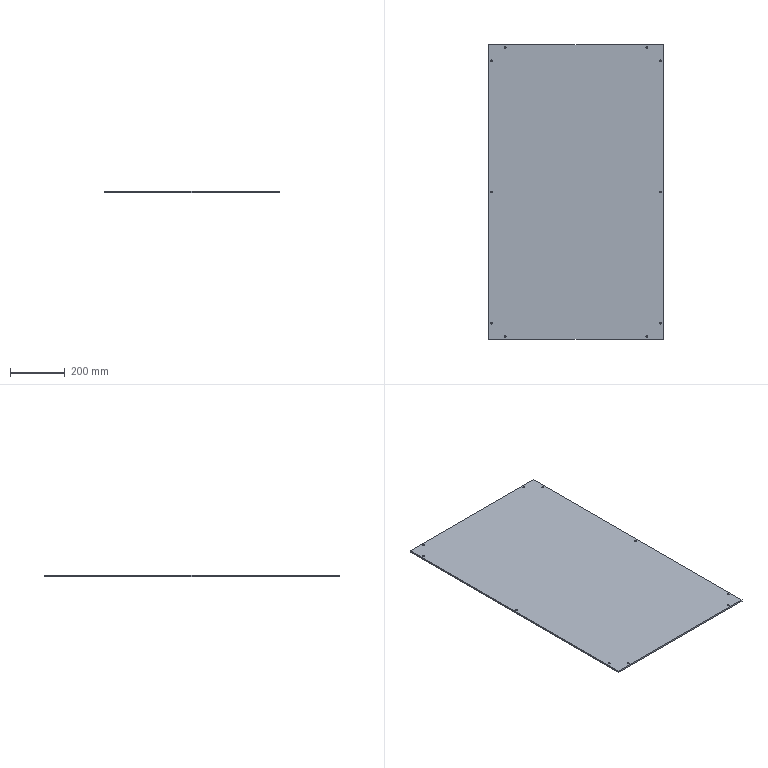Part | SolidWorks | features BaseBody 1 | 1 solid | 26 faces | box 638 x 1078 x 6 mm | volume 4124275 mm3 | cylinder 20 | plane 6 | commonest cylinder face diameters 7 x20
STEP:
#1=CARTESIAN_POINT('',(304.5,-479.,0.));
#2=VERTEX_POINT('',#1);
#3=CARTESIAN_POINT('',(311.5,-479.,0.));
#4=VERTEX_POINT('',#3);
#5=CARTESIAN_POINT('',(308.,-479.,0.));
#6=DIRECTION('',(0.,0.,1.));
#7=DIRECTION('',(1.,0.,0.));
#8=AXIS2_PLACEMENT_3D('',#5,#6,#7);
#9=CIRCLE('',#8,3.5);
#10=EDGE_CURVE('',#2,#4,#9,.T.);
#11=ORIENTED_EDGE('',*,*,#10,.F.);
#12=CARTESIAN_POINT('',(304.5,-479.,6.));
#13=VERTEX_POINT('',#12);
#14=CARTESIAN_POINT('',(304.5,-479.,6.));
#15=DIRECTION('',(0.,0.,1.));
#16=VECTOR('',#15,1000.);
#17=LINE('',#14,#16);
#18=EDGE_CURVE('',#2,#13,#17,.T.);
#19=ORIENTED_EDGE('',*,*,#18,.T.);
#20=CARTESIAN_POINT('',(311.5,-479.,6.));
#21=VERTEX_POINT('',#20);
#22=CARTESIAN_POINT('',(308.,-479.,6.));
#23=DIRECTION('',(0.,0.,1.));
#24=DIRECTION('',(1.,0.,0.));
#25=AXIS2_PLACEMENT_3D('',#22,#23,#24);
#26=CIRCLE('',#25,3.5);
#27=EDGE_CURVE('',#13,#21,#26,.T.);
#28=ORIENTED_EDGE('',*,*,#27,.T.);
#29=CARTESIAN_POINT('',(311.5,-479.,6.));
#30=DIRECTION('',(0.,0.,1.));
#31=VECTOR('',#30,1000.);
#32=LINE('',#29,#31);
#33=EDGE_CURVE('',#4,#21,#32,.T.);
#34=ORIENTED_EDGE('',*,*,#33,.F.);
#35=EDGE_LOOP('',(#11,#19,#28,#34));
#36=FACE_OUTER_BOUND('',#35,.T.);
#37=CARTESIAN_POINT('',(308.,-479.,6.));
#38=DIRECTION('',(0.,0.,1.));
#39=DIRECTION('',(1.,0.,0.));
#40=AXIS2_PLACEMENT_3D('',#37,#38,#39);
#41=CYLINDRICAL_SURFACE('',#40,3.5);
#42=ADVANCED_FACE('',(#36),#41,.F.);
#43=CARTESIAN_POINT('',(304.5,0.,0.));
#44=VERTEX_POINT('',#43);
#45=CARTESIAN_POINT('',(311.5,0.,0.));
#46=VERTEX_POINT('',#45);
#47=CARTESIAN_POINT('',(308.,0.,0.));
#48=DIRECTION('',(0.,0.,1.));
#49=DIRECTION('',(1.,0.,0.));
#50=AXIS2_PLACEMENT_3D('',#47,#48,#49);
#51=CIRCLE('',#50,3.5);
#52=EDGE_CURVE('',#44,#46,#51,.T.);
#53=ORIENTED_EDGE('',*,*,#52,.F.);
#54=CARTESIAN_POINT('',(304.5,0.,6.));
#55=VERTEX_POINT('',#54);
#56=CARTESIAN_POINT('',(304.5,0.,6.));
#57=DIRECTION('',(0.,0.,1.));
#58=VECTOR('',#57,1000.);
#59=LINE('',#56,#58);
#60=EDGE_CURVE('',#44,#55,#59,.T.);
#61=ORIENTED_EDGE('',*,*,#60,.T.);
#62=CARTESIAN_POINT('',(311.5,0.,6.));
#63=VERTEX_POINT('',#62);
#64=CARTESIAN_POINT('',(308.,0.,6.));
#65=DIRECTION('',(0.,0.,1.));
#66=DIRECTION('',(1.,0.,0.));
#67=AXIS2_PLACEMENT_3D('',#64,#65,#66);
#68=CIRCLE('',#67,3.5);
#69=EDGE_CURVE('',#55,#63,#68,.T.);
#70=ORIENTED_EDGE('',*,*,#69,.T.);
#71=CARTESIAN_POINT('',(311.5,0.,6.));
#72=DIRECTION('',(0.,0.,1.));
#73=VECTOR('',#72,1000.);
#74=LINE('',#71,#73);
#75=EDGE_CURVE('',#46,#63,#74,.T.);
#76=ORIENTED_EDGE('',*,*,#75,.F.);
#77=EDGE_LOOP('',(#53,#61,#70,#76));
#78=FACE_OUTER_BOUND('',#77,.T.);
#79=CARTESIAN_POINT('',(308.,0.,6.));
#80=DIRECTION('',(0.,0.,1.));
#81=DIRECTION('',(1.,0.,0.));
#82=AXIS2_PLACEMENT_3D('',#79,#80,#81);
#83=CYLINDRICAL_SURFACE('',#82,3.5);
#84=ADVANCED_FACE('',(#78),#83,.F.);
#85=CARTESIAN_POINT('',(304.5,479.,0.));
#86=VERTEX_POINT('',#85);
#87=CARTESIAN_POINT('',(311.5,479.,0.));
#88=VERTEX_POINT('',#87);
#89=CARTESIAN_POINT('',(308.,479.,0.));
#90=DIRECTION('',(0.,0.,1.));
#91=DIRECTION('',(1.,0.,0.));
#92=AXIS2_PLACEMENT_3D('',#89,#90,#91);
#93=CIRCLE('',#92,3.5);
#94=EDGE_CURVE('',#86,#88,#93,.T.);
#95=ORIENTED_EDGE('',*,*,#94,.F.);
#96=CARTESIAN_POINT('',(304.5,479.,6.));
#97=VERTEX_POINT('',#96);
#98=CARTESIAN_POINT('',(304.5,479.,6.));
#99=DIRECTION('',(0.,0.,1.));
#100=VECTOR('',#99,1000.);
#101=LINE('',#98,#100);
#102=EDGE_CURVE('',#86,#97,#101,.T.);
#103=ORIENTED_EDGE('',*,*,#102,.T.);
#104=CARTESIAN_POINT('',(311.5,479.,6.));
#105=VERTEX_POINT('',#104);
#106=CARTESIAN_POINT('',(308.,479.,6.));
#107=DIRECTION('',(0.,0.,1.));
#108=DIRECTION('',(1.,0.,0.));
#109=AXIS2_PLACEMENT_3D('',#106,#107,#108);
#110=CIRCLE('',#109,3.5);
#111=EDGE_CURVE('',#97,#105,#110,.T.);
#112=ORIENTED_EDGE('',*,*,#111,.T.);
#113=CARTESIAN_POINT('',(311.5,479.,6.));
#114=DIRECTION('',(0.,0.,1.));
#115=VECTOR('',#114,1000.);
#116=LINE('',#113,#115);
#117=EDGE_CURVE('',#88,#105,#116,.T.);
#118=ORIENTED_EDGE('',*,*,#117,.F.);
#119=EDGE_LOOP('',(#95,#103,#112,#118));
#120=FACE_OUTER_BOUND('',#119,.T.);
#121=CARTESIAN_POINT('',(308.,479.,6.));
#122=DIRECTION('',(0.,0.,1.));
#123=DIRECTION('',(1.,0.,0.));
#124=AXIS2_PLACEMENT_3D('',#121,#122,#123);
#125=CYLINDRICAL_SURFACE('',#124,3.5);
#126=ADVANCED_FACE('',(#120),#125,.F.);
#127=CARTESIAN_POINT('',(-311.5,-479.,0.));
#128=VERTEX_POINT('',#127);
#129=CARTESIAN_POINT('',(-304.5,-479.,0.));
#130=VERTEX_POINT('',#129);
#131=CARTESIAN_POINT('',(-308.,-479.,0.));
#132=DIRECTION('',(0.,0.,1.));
#133=DIRECTION('',(1.,0.,0.));
#134=AXIS2_PLACEMENT_3D('',#131,#132,#133);
#135=CIRCLE('',#134,3.5);
#136=EDGE_CURVE('',#128,#130,#135,.T.);
#137=ORIENTED_EDGE('',*,*,#136,.F.);
#138=CARTESIAN_POINT('',(-311.5,-479.,6.));
#139=VERTEX_POINT('',#138);
#140=CARTESIAN_POINT('',(-311.5,-479.,6.));
#141=DIRECTION('',(0.,0.,1.));
#142=VECTOR('',#141,1000.);
#143=LINE('',#140,#142);
#144=EDGE_CURVE('',#128,#139,#143,.T.);
#145=ORIENTED_EDGE('',*,*,#144,.T.);
#146=CARTESIAN_POINT('',(-304.5,-479.,6.));
#147=VERTEX_POINT('',#146);
#148=CARTESIAN_POINT('',(-308.,-479.,6.));
#149=DIRECTION('',(0.,0.,1.));
#150=DIRECTION('',(1.,0.,0.));
#151=AXIS2_PLACEMENT_3D('',#148,#149,#150);
#152=CIRCLE('',#151,3.5);
#153=EDGE_CURVE('',#139,#147,#152,.T.);
#154=ORIENTED_EDGE('',*,*,#153,.T.);
#155=CARTESIAN_POINT('',(-304.5,-479.,6.));
#156=DIRECTION('',(0.,0.,1.));
#157=VECTOR('',#156,1000.);
#158=LINE('',#155,#157);
#159=EDGE_CURVE('',#130,#147,#158,.T.);
#160=ORIENTED_EDGE('',*,*,#159,.F.);
#161=EDGE_LOOP('',(#137,#145,#154,#160));
#162=FACE_OUTER_BOUND('',#161,.T.);
#163=CARTESIAN_POINT('',(-308.,-479.,6.));
#164=DIRECTION('',(0.,0.,1.));
#165=DIRECTION('',(1.,0.,0.));
#166=AXIS2_PLACEMENT_3D('',#163,#164,#165);
#167=CYLINDRICAL_SURFACE('',#166,3.5);
#168=ADVANCED_FACE('',(#162),#167,.F.);
#169=CARTESIAN_POINT('',(-311.5,0.,0.));
#170=VERTEX_POINT('',#169);
#171=CARTESIAN_POINT('',(-304.5,0.,0.));
#172=VERTEX_POINT('',#171);
#173=CARTESIAN_POINT('',(-308.,0.,0.));
#174=DIRECTION('',(0.,0.,1.));
#175=DIRECTION('',(1.,0.,0.));
#176=AXIS2_PLACEMENT_3D('',#173,#174,#175);
#177=CIRCLE('',#176,3.5);
#178=EDGE_CURVE('',#170,#172,#177,.T.);
#179=ORIENTED_EDGE('',*,*,#178,.F.);
#180=CARTESIAN_POINT('',(-311.5,0.,6.));
#181=VERTEX_POINT('',#180);
#182=CARTESIAN_POINT('',(-311.5,0.,6.));
#183=DIRECTION('',(0.,0.,1.));
#184=VECTOR('',#183,1000.);
#185=LINE('',#182,#184);
#186=EDGE_CURVE('',#170,#181,#185,.T.);
#187=ORIENTED_EDGE('',*,*,#186,.T.);
#188=CARTESIAN_POINT('',(-304.5,0.,6.));
#189=VERTEX_POINT('',#188);
#190=CARTESIAN_POINT('',(-308.,0.,6.));
#191=DIRECTION('',(0.,0.,1.));
#192=DIRECTION('',(1.,0.,0.));
#193=AXIS2_PLACEMENT_3D('',#190,#191,#192);
#194=CIRCLE('',#193,3.5);
#195=EDGE_CURVE('',#181,#189,#194,.T.);
#196=ORIENTED_EDGE('',*,*,#195,.T.);
#197=CARTESIAN_POINT('',(-304.5,0.,6.));
#198=DIRECTION('',(0.,0.,1.));
#199=VECTOR('',#198,1000.);
#200=LINE('',#197,#199);
#201=EDGE_CURVE('',#172,#189,#200,.T.);
#202=ORIENTED_EDGE('',*,*,#201,.F.);
#203=EDGE_LOOP('',(#179,#187,#196,#202));
#204=FACE_OUTER_BOUND('',#203,.T.);
#205=CARTESIAN_POINT('',(-308.,0.,6.));
#206=DIRECTION('',(0.,0.,1.));
#207=DIRECTION('',(1.,0.,0.));
#208=AXIS2_PLACEMENT_3D('',#205,#206,#207);
#209=CYLINDRICAL_SURFACE('',#208,3.5);
#210=ADVANCED_FACE('',(#204),#209,.F.);
#211=CARTESIAN_POINT('',(255.5,-528.,0.));
#212=VERTEX_POINT('',#211);
#213=CARTESIAN_POINT('',(262.5,-528.,0.));
#214=VERTEX_POINT('',#213);
#215=CARTESIAN_POINT('',(259.,-528.,0.));
#216=DIRECTION('',(0.,0.,1.));
#217=DIRECTION('',(1.,0.,0.));
#218=AXIS2_PLACEMENT_3D('',#215,#216,#217);
#219=CIRCLE('',#218,3.5);
#220=EDGE_CURVE('',#212,#214,#219,.T.);
#221=ORIENTED_EDGE('',*,*,#220,.F.);
#222=CARTESIAN_POINT('',(255.5,-528.,6.));
#223=VERTEX_POINT('',#222);
#224=CARTESIAN_POINT('',(255.5,-528.,6.));
#225=DIRECTION('',(0.,0.,1.));
#226=VECTOR('',#225,1000.);
#227=LINE('',#224,#226);
#228=EDGE_CURVE('',#212,#223,#227,.T.);
#229=ORIENTED_EDGE('',*,*,#228,.T.);
#230=CARTESIAN_POINT('',(262.5,-528.,6.));
#231=VERTEX_POINT('',#230);
#232=CARTESIAN_POINT('',(259.,-528.,6.));
#233=DIRECTION('',(0.,0.,1.));
#234=DIRECTION('',(1.,0.,0.));
#235=AXIS2_PLACEMENT_3D('',#232,#233,#234);
#236=CIRCLE('',#235,3.5);
#237=EDGE_CURVE('',#223,#231,#236,.T.);
#238=ORIENTED_EDGE('',*,*,#237,.T.);
#239=CARTESIAN_POINT('',(262.5,-528.,6.));
#240=DIRECTION('',(0.,0.,1.));
#241=VECTOR('',#240,1000.);
#242=LINE('',#239,#241);
#243=EDGE_CURVE('',#214,#231,#242,.T.);
#244=ORIENTED_EDGE('',*,*,#243,.F.);
#245=EDGE_LOOP('',(#221,#229,#238,#244));
#246=FACE_OUTER_BOUND('',#245,.T.);
#247=CARTESIAN_POINT('',(259.,-528.,6.));
#248=DIRECTION('',(0.,0.,1.));
#249=DIRECTION('',(1.,0.,0.));
#250=AXIS2_PLACEMENT_3D('',#247,#248,#249);
#251=CYLINDRICAL_SURFACE('',#250,3.5);
#252=ADVANCED_FACE('',(#246),#251,.F.);
#253=CARTESIAN_POINT('',(-262.5,-528.,0.));
#254=VERTEX_POINT('',#253);
#255=CARTESIAN_POINT('',(-255.5,-528.,0.));
#256=VERTEX_POINT('',#255);
#257=CARTESIAN_POINT('',(-259.,-528.,0.));
#258=DIRECTION('',(0.,0.,1.));
#259=DIRECTION('',(1.,0.,0.));
#260=AXIS2_PLACEMENT_3D('',#257,#258,#259);
#261=CIRCLE('',#260,3.5);
#262=EDGE_CURVE('',#254,#256,#261,.T.);
#263=ORIENTED_EDGE('',*,*,#262,.F.);
#264=CARTESIAN_POINT('',(-262.5,-528.,6.));
#265=VERTEX_POINT('',#264);
#266=CARTESIAN_POINT('',(-262.5,-528.,6.));
#267=DIRECTION('',(0.,0.,1.));
#268=VECTOR('',#267,1000.);
#269=LINE('',#266,#268);
#270=EDGE_CURVE('',#254,#265,#269,.T.);
#271=ORIENTED_EDGE('',*,*,#270,.T.);
#272=CARTESIAN_POINT('',(-255.5,-528.,6.));
#273=VERTEX_POINT('',#272);
#274=CARTESIAN_POINT('',(-259.,-528.,6.));
#275=DIRECTION('',(0.,0.,1.));
#276=DIRECTION('',(1.,0.,0.));
#277=AXIS2_PLACEMENT_3D('',#274,#275,#276);
#278=CIRCLE('',#277,3.5);
#279=EDGE_CURVE('',#265,#273,#278,.T.);
#280=ORIENTED_EDGE('',*,*,#279,.T.);
#281=CARTESIAN_POINT('',(-255.5,-528.,6.));
#282=DIRECTION('',(0.,0.,1.));
#283=VECTOR('',#282,1000.);
#284=LINE('',#281,#283);
#285=EDGE_CURVE('',#256,#273,#284,.T.);
#286=ORIENTED_EDGE('',*,*,#285,.F.);
#287=EDGE_LOOP('',(#263,#271,#280,#286));
#288=FACE_OUTER_BOUND('',#287,.T.);
#289=CARTESIAN_POINT('',(-259.,-528.,6.));
#290=DIRECTION('',(0.,0.,1.));
#291=DIRECTION('',(1.,0.,0.));
#292=AXIS2_PLACEMENT_3D('',#289,#290,#291);
#293=CYLINDRICAL_SURFACE('',#292,3.5);
#294=ADVANCED_FACE('',(#288),#293,.F.);
#295=CARTESIAN_POINT('',(255.5,528.,0.));
#296=VERTEX_POINT('',#295);
#297=CARTESIAN_POINT('',(262.5,528.,0.));
#298=VERTEX_POINT('',#297);
#299=CARTESIAN_POINT('',(259.,528.,0.));
#300=DIRECTION('',(0.,0.,1.));
#301=DIRECTION('',(1.,0.,0.));
#302=AXIS2_PLACEMENT_3D('',#299,#300,#301);
#303=CIRCLE('',#302,3.5);
#304=EDGE_CURVE('',#296,#298,#303,.T.);
#305=ORIENTED_EDGE('',*,*,#304,.F.);
#306=CARTESIAN_POINT('',(255.5,528.,6.));
#307=VERTEX_POINT('',#306);
#308=CARTESIAN_POINT('',(255.5,528.,6.));
#309=DIRECTION('',(0.,0.,1.));
#310=VECTOR('',#309,1000.);
#311=LINE('',#308,#310);
#312=EDGE_CURVE('',#296,#307,#311,.T.);
#313=ORIENTED_EDGE('',*,*,#312,.T.);
#314=CARTESIAN_POINT('',(262.5,528.,6.));
#315=VERTEX_POINT('',#314);
#316=CARTESIAN_POINT('',(259.,528.,6.));
#317=DIRECTION('',(0.,0.,1.));
#318=DIRECTION('',(1.,0.,0.));
#319=AXIS2_PLACEMENT_3D('',#316,#317,#318);
#320=CIRCLE('',#319,3.5);
#321=EDGE_CURVE('',#307,#315,#320,.T.);
#322=ORIENTED_EDGE('',*,*,#321,.T.);
#323=CARTESIAN_POINT('',(262.5,528.,6.));
#324=DIRECTION('',(0.,0.,1.));
#325=VECTOR('',#324,1000.);
#326=LINE('',#323,#325);
#327=EDGE_CURVE('',#298,#315,#326,.T.);
#328=ORIENTED_EDGE('',*,*,#327,.F.);
#329=EDGE_LOOP('',(#305,#313,#322,#328));
#330=FACE_OUTER_BOUND('',#329,.T.);
#331=CARTESIAN_POINT('',(259.,528.,6.));
#332=DIRECTION('',(0.,0.,1.));
#333=DIRECTION('',(1.,0.,0.));
#334=AXIS2_PLACEMENT_3D('',#331,#332,#333);
#335=CYLINDRICAL_SURFACE('',#334,3.5);
#336=ADVANCED_FACE('',(#330),#335,.F.);
#337=CARTESIAN_POINT('',(-262.5,528.,0.));
#338=VERTEX_POINT('',#337);
#339=CARTESIAN_POINT('',(-255.5,528.,0.));
#340=VERTEX_POINT('',#339);
#341=CARTESIAN_POINT('',(-259.,528.,0.));
#342=DIRECTION('',(0.,0.,1.));
#343=DIRECTION('',(1.,0.,0.));
#344=AXIS2_PLACEMENT_3D('',#341,#342,#343);
#345=CIRCLE('',#344,3.5);
#346=EDGE_CURVE('',#338,#340,#345,.T.);
#347=ORIENTED_EDGE('',*,*,#346,.F.);
#348=CARTESIAN_POINT('',(-262.5,528.,6.));
#349=VERTEX_POINT('',#348);
#350=CARTESIAN_POINT('',(-262.5,528.,6.));
#351=DIRECTION('',(0.,0.,1.));
#352=VECTOR('',#351,1000.);
#353=LINE('',#350,#352);
#354=EDGE_CURVE('',#338,#349,#353,.T.);
#355=ORIENTED_EDGE('',*,*,#354,.T.);
#356=CARTESIAN_POINT('',(-255.5,528.,6.));
#357=VERTEX_POINT('',#356);
#358=CARTESIAN_POINT('',(-259.,528.,6.));
#359=DIRECTION('',(0.,0.,1.));
#360=DIRECTION('',(1.,0.,0.));
#361=AXIS2_PLACEMENT_3D('',#358,#359,#360);
#362=CIRCLE('',#361,3.5);
#363=EDGE_CURVE('',#349,#357,#362,.T.);
#364=ORIENTED_EDGE('',*,*,#363,.T.);
#365=CARTESIAN_POINT('',(-255.5,528.,6.));
#366=DIRECTION('',(0.,0.,1.));
#367=VECTOR('',#366,1000.);
#368=LINE('',#365,#367);
#369=EDGE_CURVE('',#340,#357,#368,.T.);
#370=ORIENTED_EDGE('',*,*,#369,.F.);
#371=EDGE_LOOP('',(#347,#355,#364,#370));
#372=FACE_OUTER_BOUND('',#371,.T.);
#373=CARTESIAN_POINT('',(-259.,528.,6.));
#374=DIRECTION('',(0.,0.,1.));
#375=DIRECTION('',(1.,0.,0.));
#376=AXIS2_PLACEMENT_3D('',#373,#374,#375);
#377=CYLINDRICAL_SURFACE('',#376,3.5);
#378=ADVANCED_FACE('',(#372),#377,.F.);
#379=CARTESIAN_POINT('',(-311.5,479.,0.));
#380=VERTEX_POINT('',#379);
#381=CARTESIAN_POINT('',(-304.5,479.,0.));
#382=VERTEX_POINT('',#381);
#383=CARTESIAN_POINT('',(-308.,479.,0.));
#384=DIRECTION('',(0.,0.,1.));
#385=DIRECTION('',(1.,0.,0.));
#386=AXIS2_PLACEMENT_3D('',#383,#384,#385);
#387=CIRCLE('',#386,3.5);
#388=EDGE_CURVE('',#380,#382,#387,.T.);
#389=ORIENTED_EDGE('',*,*,#388,.F.);
#390=CARTESIAN_POINT('',(-311.5,479.,6.));
#391=VERTEX_POINT('',#390);
#392=CARTESIAN_POINT('',(-311.5,479.,6.));
#393=DIRECTION('',(0.,0.,1.));
#394=VECTOR('',#393,1000.);
#395=LINE('',#392,#394);
#396=EDGE_CURVE('',#380,#391,#395,.T.);
#397=ORIENTED_EDGE('',*,*,#396,.T.);
#398=CARTESIAN_POINT('',(-304.5,479.,6.));
#399=VERTEX_POINT('',#398);
#400=CARTESIAN_POINT('',(-308.,479.,6.));
#401=DIRECTION('',(0.,0.,1.));
#402=DIRECTION('',(1.,0.,0.));
#403=AXIS2_PLACEMENT_3D('',#400,#401,#402);
#404=CIRCLE('',#403,3.5);
#405=EDGE_CURVE('',#391,#399,#404,.T.);
#406=ORIENTED_EDGE('',*,*,#405,.T.);
#407=CARTESIAN_POINT('',(-304.5,479.,6.));
#408=DIRECTION('',(0.,0.,1.));
#409=VECTOR('',#408,1000.);
#410=LINE('',#407,#409);
#411=EDGE_CURVE('',#382,#399,#410,.T.);
#412=ORIENTED_EDGE('',*,*,#411,.F.);
#413=EDGE_LOOP('',(#389,#397,#406,#412));
#414=FACE_OUTER_BOUND('',#413,.T.);
#415=CARTESIAN_POINT('',(-308.,479.,6.));
#416=DIRECTION('',(0.,0.,1.));
#417=DIRECTION('',(1.,0.,0.));
#418=AXIS2_PLACEMENT_3D('',#415,#416,#417);
#419=CYLINDRICAL_SURFACE('',#418,3.5);
#420=ADVANCED_FACE('',(#414),#419,.F.);
#421=CARTESIAN_POINT('',(308.,-479.,0.));
#422=DIRECTION('',(0.,0.,1.));
#423=DIRECTION('',(1.,0.,0.));
#424=AXIS2_PLACEMENT_3D('',#421,#422,#423);
#425=CIRCLE('',#424,3.5);
#426=EDGE_CURVE('',#4,#2,#425,.T.);
#427=ORIENTED_EDGE('',*,*,#426,.T.);
#428=ORIENTED_EDGE('',*,*,#10,.T.);
#429=EDGE_LOOP('',(#427,#428));
#430=FACE_BOUND('',#429,.T.);
#431=CARTESIAN_POINT('',(308.,0.,0.));
#432=DIRECTION('',(0.,0.,1.));
#433=DIRECTION('',(1.,0.,0.));
#434=AXIS2_PLACEMENT_3D('',#431,#432,#433);
#435=CIRCLE('',#434,3.5);
#436=EDGE_CURVE('',#46,#44,#435,.T.);
#437=ORIENTED_EDGE('',*,*,#436,.T.);
#438=ORIENTED_EDGE('',*,*,#52,.T.);
#439=EDGE_LOOP('',(#437,#438));
#440=FACE_BOUND('',#439,.T.);
#441=CARTESIAN_POINT('',(308.,479.,0.));
#442=DIRECTION('',(0.,0.,1.));
#443=DIRECTION('',(1.,0.,0.));
#444=AXIS2_PLACEMENT_3D('',#441,#442,#443);
#445=CIRCLE('',#444,3.5);
#446=EDGE_CURVE('',#88,#86,#445,.T.);
#447=ORIENTED_EDGE('',*,*,#446,.T.);
#448=ORIENTED_EDGE('',*,*,#94,.T.);
#449=EDGE_LOOP('',(#447,#448));
#450=FACE_BOUND('',#449,.T.);
#451=CARTESIAN_POINT('',(-308.,-479.,0.));
#452=DIRECTION('',(0.,0.,1.));
#453=DIRECTION('',(1.,0.,0.));
#454=AXIS2_PLACEMENT_3D('',#451,#452,#453);
#455=CIRCLE('',#454,3.5);
#456=EDGE_CURVE('',#130,#128,#455,.T.);
#457=ORIENTED_EDGE('',*,*,#456,.T.);
#458=ORIENTED_EDGE('',*,*,#136,.T.);
#459=EDGE_LOOP('',(#457,#458));
#460=FACE_BOUND('',#459,.T.);
#461=CARTESIAN_POINT('',(259.,-528.,0.));
#462=DIRECTION('',(0.,0.,1.));
#463=DIRECTION('',(1.,0.,0.));
#464=AXIS2_PLACEMENT_3D('',#461,#462,#463);
#465=CIRCLE('',#464,3.5);
#466=EDGE_CURVE('',#214,#212,#465,.T.);
#467=ORIENTED_EDGE('',*,*,#466,.T.);
#468=ORIENTED_EDGE('',*,*,#220,.T.);
#469=EDGE_LOOP('',(#467,#468));
#470=FACE_BOUND('',#469,.T.);
#471=CARTESIAN_POINT('',(-259.,-528.,0.));
#472=DIRECTION('',(0.,0.,1.));
#473=DIRECTION('',(1.,0.,0.));
#474=AXIS2_PLACEMENT_3D('',#471,#472,#473);
#475=CIRCLE('',#474,3.5);
#476=EDGE_CURVE('',#256,#254,#475,.T.);
#477=ORIENTED_EDGE('',*,*,#476,.T.);
#478=ORIENTED_EDGE('',*,*,#262,.T.);
#479=EDGE_LOOP('',(#477,#478));
#480=FACE_BOUND('',#479,.T.);
#481=CARTESIAN_POINT('',(-308.,479.,0.));
#482=DIRECTION('',(0.,0.,1.));
#483=DIRECTION('',(1.,0.,0.));
#484=AXIS2_PLACEMENT_3D('',#481,#482,#483);
#485=CIRCLE('',#484,3.5);
#486=EDGE_CURVE('',#382,#380,#485,.T.);
#487=ORIENTED_EDGE('',*,*,#486,.T.);
#488=ORIENTED_EDGE('',*,*,#388,.T.);
#489=EDGE_LOOP('',(#487,#488));
#490=FACE_BOUND('',#489,.T.);
#491=CARTESIAN_POINT('',(-259.,528.,0.));
#492=DIRECTION('',(0.,0.,1.));
#493=DIRECTION('',(1.,0.,0.));
#494=AXIS2_PLACEMENT_3D('',#491,#492,#493);
#495=CIRCLE('',#494,3.5);
#496=EDGE_CURVE('',#340,#338,#495,.T.);
#497=ORIENTED_EDGE('',*,*,#496,.T.);
#498=ORIENTED_EDGE('',*,*,#346,.T.);
#499=EDGE_LOOP('',(#497,#498));
#500=FACE_BOUND('',#499,.T.);
#501=CARTESIAN_POINT('',(259.,528.,0.));
#502=DIRECTION('',(0.,0.,1.));
#503=DIRECTION('',(1.,0.,0.));
#504=AXIS2_PLACEMENT_3D('',#501,#502,#503);
#505=CIRCLE('',#504,3.5);
#506=EDGE_CURVE('',#298,#296,#505,.T.);
#507=ORIENTED_EDGE('',*,*,#506,.T.);
#508=ORIENTED_EDGE('',*,*,#304,.T.);
#509=EDGE_LOOP('',(#507,#508));
#510=FACE_BOUND('',#509,.T.);
#511=CARTESIAN_POINT('',(-308.,0.,0.));
#512=DIRECTION('',(0.,0.,1.));
#513=DIRECTION('',(1.,0.,0.));
#514=AXIS2_PLACEMENT_3D('',#511,#512,#513);
#515=CIRCLE('',#514,3.5);
#516=EDGE_CURVE('',#172,#170,#515,.T.);
#517=ORIENTED_EDGE('',*,*,#516,.T.);
#518=ORIENTED_EDGE('',*,*,#178,.T.);
#519=EDGE_LOOP('',(#517,#518));
#520=FACE_BOUND('',#519,.T.);
#521=CARTESIAN_POINT('',(319.,-539.,0.));
#522=VERTEX_POINT('',#521);
#523=CARTESIAN_POINT('',(319.,539.,0.));
#524=VERTEX_POINT('',#523);
#525=CARTESIAN_POINT('',(319.,539.,0.));
#526=DIRECTION('',(0.,1.,0.));
#527=VECTOR('',#526,1000.);
#528=LINE('',#525,#527);
#529=EDGE_CURVE('',#522,#524,#528,.T.);
#530=ORIENTED_EDGE('',*,*,#529,.F.);
#531=CARTESIAN_POINT('',(-319.,-539.,0.));
#532=VERTEX_POINT('',#531);
#533=CARTESIAN_POINT('',(-319.,-539.,0.));
#534=DIRECTION('',(1.,0.,0.));
#535=VECTOR('',#534,1000.);
#536=LINE('',#533,#535);
#537=EDGE_CURVE('',#532,#522,#536,.T.);
#538=ORIENTED_EDGE('',*,*,#537,.F.);
#539=CARTESIAN_POINT('',(-319.,539.,0.));
#540=VERTEX_POINT('',#539);
#541=CARTESIAN_POINT('',(-319.,539.,0.));
#542=DIRECTION('',(0.,-1.,0.));
#543=VECTOR('',#542,1000.);
#544=LINE('',#541,#543);
#545=EDGE_CURVE('',#540,#532,#544,.T.);
#546=ORIENTED_EDGE('',*,*,#545,.F.);
#547=CARTESIAN_POINT('',(-319.,539.,0.));
#548=DIRECTION('',(-1.,0.,0.));
#549=VECTOR('',#548,1000.);
#550=LINE('',#547,#549);
#551=EDGE_CURVE('',#524,#540,#550,.T.);
#552=ORIENTED_EDGE('',*,*,#551,.F.);
#553=EDGE_LOOP('',(#530,#538,#546,#552));
#554=FACE_OUTER_BOUND('',#553,.T.);
#555=CARTESIAN_POINT('',(0.,0.,0.));
#556=DIRECTION('',(0.,0.,1.));
#557=DIRECTION('',(1.,0.,0.));
#558=AXIS2_PLACEMENT_3D('',#555,#556,#557);
#559=PLANE('',#558);
#560=ADVANCED_FACE('',(#430,#440,#450,#460,#470,#480,#490,#500,#510,#520,#554),#559,.F.);
#561=CARTESIAN_POINT('',(308.,-479.,6.));
#562=DIRECTION('',(0.,0.,1.));
#563=DIRECTION('',(1.,0.,0.));
#564=AXIS2_PLACEMENT_3D('',#561,#562,#563);
#565=CIRCLE('',#564,3.5);
#566=EDGE_CURVE('',#21,#13,#565,.T.);
#567=ORIENTED_EDGE('',*,*,#566,.F.);
#568=ORIENTED_EDGE('',*,*,#27,.F.);
#569=EDGE_LOOP('',(#567,#568));
#570=FACE_BOUND('',#569,.T.);
#571=CARTESIAN_POINT('',(308.,0.,6.));
#572=DIRECTION('',(0.,0.,1.));
#573=DIRECTION('',(1.,0.,0.));
#574=AXIS2_PLACEMENT_3D('',#571,#572,#573);
#575=CIRCLE('',#574,3.5);
#576=EDGE_CURVE('',#63,#55,#575,.T.);
#577=ORIENTED_EDGE('',*,*,#576,.F.);
#578=ORIENTED_EDGE('',*,*,#69,.F.);
#579=EDGE_LOOP('',(#577,#578));
#580=FACE_BOUND('',#579,.T.);
#581=CARTESIAN_POINT('',(308.,479.,6.));
#582=DIRECTION('',(0.,0.,1.));
#583=DIRECTION('',(1.,0.,0.));
#584=AXIS2_PLACEMENT_3D('',#581,#582,#583);
#585=CIRCLE('',#584,3.5);
#586=EDGE_CURVE('',#105,#97,#585,.T.);
#587=ORIENTED_EDGE('',*,*,#586,.F.);
#588=ORIENTED_EDGE('',*,*,#111,.F.);
#589=EDGE_LOOP('',(#587,#588));
#590=FACE_BOUND('',#589,.T.);
#591=CARTESIAN_POINT('',(-308.,-479.,6.));
#592=DIRECTION('',(0.,0.,1.));
#593=DIRECTION('',(1.,0.,0.));
#594=AXIS2_PLACEMENT_3D('',#591,#592,#593);
#595=CIRCLE('',#594,3.5);
#596=EDGE_CURVE('',#147,#139,#595,.T.);
#597=ORIENTED_EDGE('',*,*,#596,.F.);
#598=ORIENTED_EDGE('',*,*,#153,.F.);
#599=EDGE_LOOP('',(#597,#598));
#600=FACE_BOUND('',#599,.T.);
#601=CARTESIAN_POINT('',(259.,-528.,6.));
#602=DIRECTION('',(0.,0.,1.));
#603=DIRECTION('',(1.,0.,0.));
#604=AXIS2_PLACEMENT_3D('',#601,#602,#603);
#605=CIRCLE('',#604,3.5);
#606=EDGE_CURVE('',#231,#223,#605,.T.);
#607=ORIENTED_EDGE('',*,*,#606,.F.);
#608=ORIENTED_EDGE('',*,*,#237,.F.);
#609=EDGE_LOOP('',(#607,#608));
#610=FACE_BOUND('',#609,.T.);
#611=CARTESIAN_POINT('',(-259.,-528.,6.));
#612=DIRECTION('',(0.,0.,1.));
#613=DIRECTION('',(1.,0.,0.));
#614=AXIS2_PLACEMENT_3D('',#611,#612,#613);
#615=CIRCLE('',#614,3.5);
#616=EDGE_CURVE('',#273,#265,#615,.T.);
#617=ORIENTED_EDGE('',*,*,#616,.F.);
#618=ORIENTED_EDGE('',*,*,#279,.F.);
#619=EDGE_LOOP('',(#617,#618));
#620=FACE_BOUND('',#619,.T.);
#621=CARTESIAN_POINT('',(-308.,479.,6.));
#622=DIRECTION('',(0.,0.,1.));
#623=DIRECTION('',(1.,0.,0.));
#624=AXIS2_PLACEMENT_3D('',#621,#622,#623);
#625=CIRCLE('',#624,3.5);
#626=EDGE_CURVE('',#399,#391,#625,.T.);
#627=ORIENTED_EDGE('',*,*,#626,.F.);
#628=ORIENTED_EDGE('',*,*,#405,.F.);
#629=EDGE_LOOP('',(#627,#628));
#630=FACE_BOUND('',#629,.T.);
#631=CARTESIAN_POINT('',(-259.,528.,6.));
#632=DIRECTION('',(0.,0.,1.));
#633=DIRECTION('',(1.,0.,0.));
#634=AXIS2_PLACEMENT_3D('',#631,#632,#633);
#635=CIRCLE('',#634,3.5);
#636=EDGE_CURVE('',#357,#349,#635,.T.);
#637=ORIENTED_EDGE('',*,*,#636,.F.);
#638=ORIENTED_EDGE('',*,*,#363,.F.);
#639=EDGE_LOOP('',(#637,#638));
#640=FACE_BOUND('',#639,.T.);
#641=CARTESIAN_POINT('',(259.,528.,6.));
#642=DIRECTION('',(0.,0.,1.));
#643=DIRECTION('',(1.,0.,0.));
#644=AXIS2_PLACEMENT_3D('',#641,#642,#643);
#645=CIRCLE('',#644,3.5);
#646=EDGE_CURVE('',#315,#307,#645,.T.);
#647=ORIENTED_EDGE('',*,*,#646,.F.);
#648=ORIENTED_EDGE('',*,*,#321,.F.);
#649=EDGE_LOOP('',(#647,#648));
#650=FACE_BOUND('',#649,.T.);
#651=CARTESIAN_POINT('',(-308.,0.,6.));
#652=DIRECTION('',(0.,0.,1.));
#653=DIRECTION('',(1.,0.,0.));
#654=AXIS2_PLACEMENT_3D('',#651,#652,#653);
#655=CIRCLE('',#654,3.5);
#656=EDGE_CURVE('',#189,#181,#655,.T.);
#657=ORIENTED_EDGE('',*,*,#656,.F.);
#658=ORIENTED_EDGE('',*,*,#195,.F.);
#659=EDGE_LOOP('',(#657,#658));
#660=FACE_BOUND('',#659,.T.);
#661=CARTESIAN_POINT('',(319.,-539.,6.));
#662=VERTEX_POINT('',#661);
#663=CARTESIAN_POINT('',(319.,539.,6.));
#664=VERTEX_POINT('',#663);
#665=CARTESIAN_POINT('',(319.,539.,6.));
#666=DIRECTION('',(0.,1.,0.));
#667=VECTOR('',#666,1000.);
#668=LINE('',#665,#667);
#669=EDGE_CURVE('',#662,#664,#668,.T.);
#670=ORIENTED_EDGE('',*,*,#669,.T.);
#671=CARTESIAN_POINT('',(-319.,539.,6.));
#672=VERTEX_POINT('',#671);
#673=CARTESIAN_POINT('',(-319.,539.,6.));
#674=DIRECTION('',(-1.,0.,0.));
#675=VECTOR('',#674,1000.);
#676=LINE('',#673,#675);
#677=EDGE_CURVE('',#664,#672,#676,.T.);
#678=ORIENTED_EDGE('',*,*,#677,.T.);
#679=CARTESIAN_POINT('',(-319.,-539.,6.));
#680=VERTEX_POINT('',#679);
#681=CARTESIAN_POINT('',(-319.,539.,6.));
#682=DIRECTION('',(0.,-1.,0.));
#683=VECTOR('',#682,1000.);
#684=LINE('',#681,#683);
#685=EDGE_CURVE('',#672,#680,#684,.T.);
#686=ORIENTED_EDGE('',*,*,#685,.T.);
#687=CARTESIAN_POINT('',(-319.,-539.,6.));
#688=DIRECTION('',(1.,0.,0.));
#689=VECTOR('',#688,1000.);
#690=LINE('',#687,#689);
#691=EDGE_CURVE('',#680,#662,#690,.T.);
#692=ORIENTED_EDGE('',*,*,#691,.T.);
#693=EDGE_LOOP('',(#670,#678,#686,#692));
#694=FACE_OUTER_BOUND('',#693,.T.);
#695=CARTESIAN_POINT('',(0.,0.,6.));
#696=DIRECTION('',(0.,0.,1.));
#697=DIRECTION('',(1.,0.,0.));
#698=AXIS2_PLACEMENT_3D('',#695,#696,#697);
#699=PLANE('',#698);
#700=ADVANCED_FACE('',(#570,#580,#590,#600,#610,#620,#630,#640,#650,#660,#694),#699,.T.);
#701=ORIENTED_EDGE('',*,*,#537,.T.);
#702=CARTESIAN_POINT('',(319.,-539.,6.));
#703=DIRECTION('',(0.,0.,-1.));
#704=VECTOR('',#703,1000.);
#705=LINE('',#702,#704);
#706=EDGE_CURVE('',#662,#522,#705,.T.);
#707=ORIENTED_EDGE('',*,*,#706,.F.);
#708=ORIENTED_EDGE('',*,*,#691,.F.);
#709=CARTESIAN_POINT('',(-319.,-539.,6.));
#710=DIRECTION('',(0.,0.,-1.));
#711=VECTOR('',#710,1000.);
#712=LINE('',#709,#711);
#713=EDGE_CURVE('',#680,#532,#712,.T.);
#714=ORIENTED_EDGE('',*,*,#713,.T.);
#715=EDGE_LOOP('',(#701,#707,#708,#714));
#716=FACE_OUTER_BOUND('',#715,.T.);
#717=CARTESIAN_POINT('',(-319.,-539.,6.));
#718=DIRECTION('',(0.,1.,0.));
#719=DIRECTION('',(1.,0.,0.));
#720=AXIS2_PLACEMENT_3D('',#717,#718,#719);
#721=PLANE('',#720);
#722=ADVANCED_FACE('',(#716),#721,.F.);
#723=ORIENTED_EDGE('',*,*,#545,.T.);
#724=ORIENTED_EDGE('',*,*,#713,.F.);
#725=ORIENTED_EDGE('',*,*,#685,.F.);
#726=CARTESIAN_POINT('',(-319.,539.,6.));
#727=DIRECTION('',(0.,0.,-1.));
#728=VECTOR('',#727,1000.);
#729=LINE('',#726,#728);
#730=EDGE_CURVE('',#672,#540,#729,.T.);
#731=ORIENTED_EDGE('',*,*,#730,.T.);
#732=EDGE_LOOP('',(#723,#724,#725,#731));
#733=FACE_OUTER_BOUND('',#732,.T.);
#734=CARTESIAN_POINT('',(-319.,539.,6.));
#735=DIRECTION('',(1.,0.,0.));
#736=DIRECTION('',(0.,1.,0.));
#737=AXIS2_PLACEMENT_3D('',#734,#735,#736);
#738=PLANE('',#737);
#739=ADVANCED_FACE('',(#733),#738,.F.);
#740=ORIENTED_EDGE('',*,*,#551,.T.);
#741=ORIENTED_EDGE('',*,*,#730,.F.);
#742=ORIENTED_EDGE('',*,*,#677,.F.);
#743=CARTESIAN_POINT('',(319.,539.,6.));
#744=DIRECTION('',(0.,0.,-1.));
#745=VECTOR('',#744,1000.);
#746=LINE('',#743,#745);
#747=EDGE_CURVE('',#664,#524,#746,.T.);
#748=ORIENTED_EDGE('',*,*,#747,.T.);
#749=EDGE_LOOP('',(#740,#741,#742,#748));
#750=FACE_OUTER_BOUND('',#749,.T.);
#751=CARTESIAN_POINT('',(-319.,539.,6.));
#752=DIRECTION('',(0.,-1.,0.));
#753=DIRECTION('',(0.,0.,-1.));
#754=AXIS2_PLACEMENT_3D('',#751,#752,#753);
#755=PLANE('',#754);
#756=ADVANCED_FACE('',(#750),#755,.F.);
#757=ORIENTED_EDGE('',*,*,#529,.T.);
#758=ORIENTED_EDGE('',*,*,#747,.F.);
#759=ORIENTED_EDGE('',*,*,#669,.F.);
#760=ORIENTED_EDGE('',*,*,#706,.T.);
#761=EDGE_LOOP('',(#757,#758,#759,#760));
#762=FACE_OUTER_BOUND('',#761,.T.);
#763=CARTESIAN_POINT('',(319.,539.,6.));
#764=DIRECTION('',(-1.,0.,0.));
#765=DIRECTION('',(0.,1.,0.));
#766=AXIS2_PLACEMENT_3D('',#763,#764,#765);
#767=PLANE('',#766);
#768=ADVANCED_FACE('',(#762),#767,.F.);
#769=ORIENTED_EDGE('',*,*,#396,.F.);
#770=ORIENTED_EDGE('',*,*,#486,.F.);
#771=ORIENTED_EDGE('',*,*,#411,.T.);
#772=ORIENTED_EDGE('',*,*,#626,.T.);
#773=EDGE_LOOP('',(#769,#770,#771,#772));
#774=FACE_OUTER_BOUND('',#773,.T.);
#775=CARTESIAN_POINT('',(-308.,479.,6.));
#776=DIRECTION('',(0.,0.,1.));
#777=DIRECTION('',(1.,0.,0.));
#778=AXIS2_PLACEMENT_3D('',#775,#776,#777);
#779=CYLINDRICAL_SURFACE('',#778,3.5);
#780=ADVANCED_FACE('',(#774),#779,.F.);
#781=ORIENTED_EDGE('',*,*,#354,.F.);
#782=ORIENTED_EDGE('',*,*,#496,.F.);
#783=ORIENTED_EDGE('',*,*,#369,.T.);
#784=ORIENTED_EDGE('',*,*,#636,.T.);
#785=EDGE_LOOP('',(#781,#782,#783,#784));
#786=FACE_OUTER_BOUND('',#785,.T.);
#787=CARTESIAN_POINT('',(-259.,528.,6.));
#788=DIRECTION('',(0.,0.,1.));
#789=DIRECTION('',(1.,0.,0.));
#790=AXIS2_PLACEMENT_3D('',#787,#788,#789);
#791=CYLINDRICAL_SURFACE('',#790,3.5);
#792=ADVANCED_FACE('',(#786),#791,.F.);
#793=ORIENTED_EDGE('',*,*,#312,.F.);
#794=ORIENTED_EDGE('',*,*,#506,.F.);
#795=ORIENTED_EDGE('',*,*,#327,.T.);
#796=ORIENTED_EDGE('',*,*,#646,.T.);
#797=EDGE_LOOP('',(#793,#794,#795,#796));
#798=FACE_OUTER_BOUND('',#797,.T.);
#799=CARTESIAN_POINT('',(259.,528.,6.));
#800=DIRECTION('',(0.,0.,1.));
#801=DIRECTION('',(1.,0.,0.));
#802=AXIS2_PLACEMENT_3D('',#799,#800,#801);
#803=CYLINDRICAL_SURFACE('',#802,3.5);
#804=ADVANCED_FACE('',(#798),#803,.F.);
#805=ORIENTED_EDGE('',*,*,#270,.F.);
#806=ORIENTED_EDGE('',*,*,#476,.F.);
#807=ORIENTED_EDGE('',*,*,#285,.T.);
#808=ORIENTED_EDGE('',*,*,#616,.T.);
#809=EDGE_LOOP('',(#805,#806,#807,#808));
#810=FACE_OUTER_BOUND('',#809,.T.);
#811=CARTESIAN_POINT('',(-259.,-528.,6.));
#812=DIRECTION('',(0.,0.,1.));
#813=DIRECTION('',(1.,0.,0.));
#814=AXIS2_PLACEMENT_3D('',#811,#812,#813);
#815=CYLINDRICAL_SURFACE('',#814,3.5);
#816=ADVANCED_FACE('',(#810),#815,.F.);
#817=ORIENTED_EDGE('',*,*,#228,.F.);
#818=ORIENTED_EDGE('',*,*,#466,.F.);
#819=ORIENTED_EDGE('',*,*,#243,.T.);
#820=ORIENTED_EDGE('',*,*,#606,.T.);
#821=EDGE_LOOP('',(#817,#818,#819,#820));
#822=FACE_OUTER_BOUND('',#821,.T.);
#823=CARTESIAN_POINT('',(259.,-528.,6.));
#824=DIRECTION('',(0.,0.,1.));
#825=DIRECTION('',(1.,0.,0.));
#826=AXIS2_PLACEMENT_3D('',#823,#824,#825);
#827=CYLINDRICAL_SURFACE('',#826,3.5);
#828=ADVANCED_FACE('',(#822),#827,.F.);
#829=ORIENTED_EDGE('',*,*,#186,.F.);
#830=ORIENTED_EDGE('',*,*,#516,.F.);
#831=ORIENTED_EDGE('',*,*,#201,.T.);
#832=ORIENTED_EDGE('',*,*,#656,.T.);
#833=EDGE_LOOP('',(#829,#830,#831,#832));
#834=FACE_OUTER_BOUND('',#833,.T.);
#835=CARTESIAN_POINT('',(-308.,0.,6.));
#836=DIRECTION('',(0.,0.,1.));
#837=DIRECTION('',(1.,0.,0.));
#838=AXIS2_PLACEMENT_3D('',#835,#836,#837);
#839=CYLINDRICAL_SURFACE('',#838,3.5);
#840=ADVANCED_FACE('',(#834),#839,.F.);
#841=ORIENTED_EDGE('',*,*,#144,.F.);
#842=ORIENTED_EDGE('',*,*,#456,.F.);
#843=ORIENTED_EDGE('',*,*,#159,.T.);
#844=ORIENTED_EDGE('',*,*,#596,.T.);
#845=EDGE_LOOP('',(#841,#842,#843,#844));
#846=FACE_OUTER_BOUND('',#845,.T.);
#847=CARTESIAN_POINT('',(-308.,-479.,6.));
#848=DIRECTION('',(0.,0.,1.));
#849=DIRECTION('',(1.,0.,0.));
#850=AXIS2_PLACEMENT_3D('',#847,#848,#849);
#851=CYLINDRICAL_SURFACE('',#850,3.5);
#852=ADVANCED_FACE('',(#846),#851,.F.);
#853=ORIENTED_EDGE('',*,*,#102,.F.);
#854=ORIENTED_EDGE('',*,*,#446,.F.);
#855=ORIENTED_EDGE('',*,*,#117,.T.);
#856=ORIENTED_EDGE('',*,*,#586,.T.);
#857=EDGE_LOOP('',(#853,#854,#855,#856));
#858=FACE_OUTER_BOUND('',#857,.T.);
#859=CARTESIAN_POINT('',(308.,479.,6.));
#860=DIRECTION('',(0.,0.,1.));
#861=DIRECTION('',(1.,0.,0.));
#862=AXIS2_PLACEMENT_3D('',#859,#860,#861);
#863=CYLINDRICAL_SURFACE('',#862,3.5);
#864=ADVANCED_FACE('',(#858),#863,.F.);
#865=ORIENTED_EDGE('',*,*,#60,.F.);
#866=ORIENTED_EDGE('',*,*,#436,.F.);
#867=ORIENTED_EDGE('',*,*,#75,.T.);
#868=ORIENTED_EDGE('',*,*,#576,.T.);
#869=EDGE_LOOP('',(#865,#866,#867,#868));
#870=FACE_OUTER_BOUND('',#869,.T.);
#871=CARTESIAN_POINT('',(308.,0.,6.));
#872=DIRECTION('',(0.,0.,1.));
#873=DIRECTION('',(1.,0.,0.));
#874=AXIS2_PLACEMENT_3D('',#871,#872,#873);
#875=CYLINDRICAL_SURFACE('',#874,3.5);
#876=ADVANCED_FACE('',(#870),#875,.F.);
#877=ORIENTED_EDGE('',*,*,#18,.F.);
#878=ORIENTED_EDGE('',*,*,#426,.F.);
#879=ORIENTED_EDGE('',*,*,#33,.T.);
#880=ORIENTED_EDGE('',*,*,#566,.T.);
#881=EDGE_LOOP('',(#877,#878,#879,#880));
#882=FACE_OUTER_BOUND('',#881,.T.);
#883=CARTESIAN_POINT('',(308.,-479.,6.));
#884=DIRECTION('',(0.,0.,1.));
#885=DIRECTION('',(1.,0.,0.));
#886=AXIS2_PLACEMENT_3D('',#883,#884,#885);
#887=CYLINDRICAL_SURFACE('',#886,3.5);
#888=ADVANCED_FACE('',(#882),#887,.F.);
#889=CLOSED_SHELL('',(#42,#84,#126,#168,#210,#252,#294,#336,#378,#420,#560,#700,#722,#739,#756,#768,#780,#792,#804,#816,#828,#840,#852,#864,#876,#888));
#890=MANIFOLD_SOLID_BREP('',#889);
#891=CARTESIAN_POINT('',(0.,0.,0.));
#892=DIRECTION('',(0.,0.,1.));
#893=DIRECTION('',(1.,0.,0.));
#894=AXIS2_PLACEMENT_3D('',#891,#892,#893);
#895=(LENGTH_UNIT()NAMED_UNIT(*)SI_UNIT(.MILLI.,.METRE.));
#896=UNCERTAINTY_MEASURE_WITH_UNIT(LENGTH_MEASURE(0.00001),#895,'','');
#897=(NAMED_UNIT(*)PLANE_ANGLE_UNIT()SI_UNIT($,.RADIAN.));
#898=(NAMED_UNIT(*)SI_UNIT($,.STERADIAN.)SOLID_ANGLE_UNIT());
#899=(GEOMETRIC_REPRESENTATION_CONTEXT(3)GLOBAL_UNCERTAINTY_ASSIGNED_CONTEXT((#896))GLOBAL_UNIT_ASSIGNED_CONTEXT((#895,#897,#898))REPRESENTATION_CONTEXT('',''));
#900=ADVANCED_BREP_SHAPE_REPRESENTATION('',(#890,#894),#899);